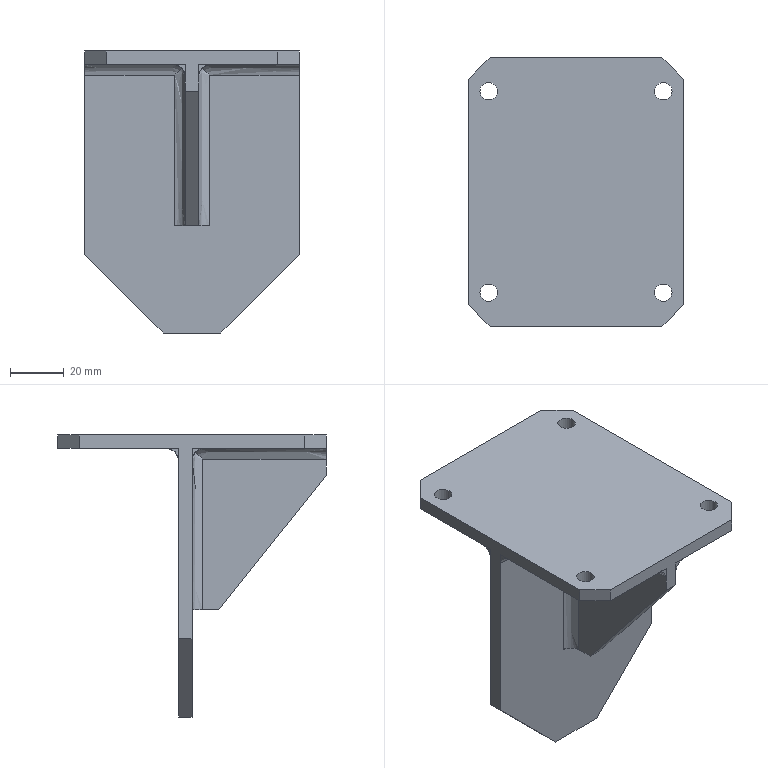Part | NX | features FILLET_WELD 5, FSET 5, EXTRUDE 3, DATUM_CSYS 2, MOVE_FACE 2, UNITE 2, CHAMFER 1, SKETCH 1 | 4 solids | 48 faces | box 80 x 100 x 105 mm | volume 85942 mm3 | plane 37 | spline 7 | cylinder 4 | commonest cylinder face diameters 6.5 x4